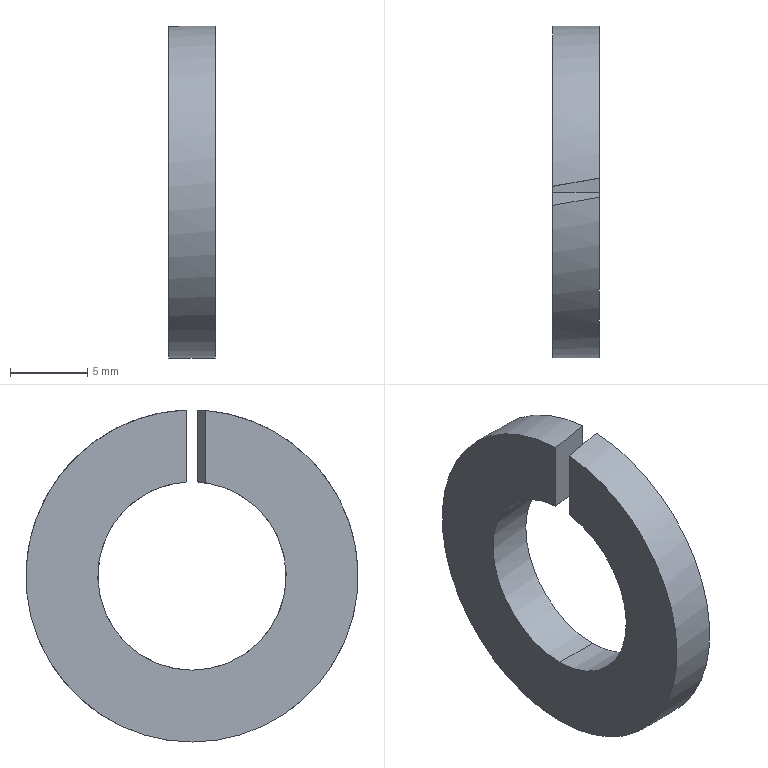Part | STEP file | 0228_318_SSLW12 | 1 solid | 8 faces | box 3 x 21.5 x 21.494 mm | volume 721.153 mm3 | cylinder 4 | plane 4 | commonest cylinder face diameters 12.2 x2 21.5 x2
STEP:
#1=CARTESIAN_POINT('',(0.,0.,0.));
#2=DIRECTION('',(0.,0.,1.));
#3=DIRECTION('',(1.,0.,0.));
#4=AXIS2_PLACEMENT_3D('',#1,#2,#3);
#5=CARTESIAN_POINT('',(-1.5,0.3549,6.09));
#6=VERTEX_POINT('',#5);
#7=CARTESIAN_POINT('',(1.5,0.8839,6.036));
#8=VERTEX_POINT('',#7);
#9=CARTESIAN_POINT('',(-1.5,0.3549,6.09));
#10=CARTESIAN_POINT('',(-0.4959,0.532,6.079));
#11=CARTESIAN_POINT('',(0.5048,0.7084,6.061));
#12=CARTESIAN_POINT('',(1.5,0.8839,6.036));
#13=(BOUNDED_CURVE()B_SPLINE_CURVE(3,(#9,#10,#11,#12),.UNSPECIFIED.,.F.,.F.)B_SPLINE_CURVE_WITH_KNOTS((4,4),(4.771,4.858),.PIECEWISE_BEZIER_KNOTS.)CURVE()GEOMETRIC_REPRESENTATION_ITEM()RATIONAL_B_SPLINE_CURVE((1.,0.9994,0.9994,1.))REPRESENTATION_ITEM(''));
#14=CARTESIAN_POINT('',(0.,0.,0.));
#15=DIRECTION('',(1.,0.,0.));
#16=DIRECTION('',(0.,0.,-1.));
#17=AXIS2_PLACEMENT_3D('',#14,#15,#16);
#18=CYLINDRICAL_SURFACE('',#17,6.1);
#19=CARTESIAN_POINT('',(3.083,-1.5));
#20=CARTESIAN_POINT('',(3.082,-1.454));
#21=CARTESIAN_POINT('',(3.079,-1.363));
#22=CARTESIAN_POINT('',(3.075,-1.226));
#23=CARTESIAN_POINT('',(3.071,-1.09));
#24=CARTESIAN_POINT('',(3.068,-0.9528));
#25=CARTESIAN_POINT('',(3.064,-0.8161));
#26=CARTESIAN_POINT('',(3.06,-0.6794));
#27=CARTESIAN_POINT('',(3.056,-0.5428));
#28=CARTESIAN_POINT('',(3.052,-0.4062));
#29=CARTESIAN_POINT('',(3.048,-0.2696));
#30=CARTESIAN_POINT('',(3.044,-0.1331));
#31=CARTESIAN_POINT('',(3.04,0.003351));
#32=CARTESIAN_POINT('',(3.036,0.1398));
#33=CARTESIAN_POINT('',(3.032,0.2761));
#34=CARTESIAN_POINT('',(3.028,0.4124));
#35=CARTESIAN_POINT('',(3.024,0.5486));
#36=CARTESIAN_POINT('',(3.02,0.6847));
#37=CARTESIAN_POINT('',(3.016,0.8208));
#38=CARTESIAN_POINT('',(3.012,0.9568));
#39=CARTESIAN_POINT('',(3.008,1.093));
#40=CARTESIAN_POINT('',(3.004,1.229));
#41=CARTESIAN_POINT('',(3.,1.364));
#42=CARTESIAN_POINT('',(2.997,1.455));
#43=CARTESIAN_POINT('',(2.996,1.5));
#44=B_SPLINE_CURVE_WITH_KNOTS('',3,(#19,#20,#21,#22,#23,#24,#25,#26,#27,#28,#29,#30,#31,#32,#33,#34,#35,#36,#37,#38,#39,#40,#41,#42,#43),.UNSPECIFIED.,.F.,.F.,(4,1,1,1,1,1,1,1,1,1,1,1,1,1,1,1,1,1,1,1,1,1,4),(4.771,4.775,4.779,4.782,4.786,4.79,4.794,4.798,4.802,4.806,4.81,4.814,4.818,4.822,4.826,4.83,4.834,4.838,4.842,4.846,4.85,4.854,4.858),.QUASI_UNIFORM_KNOTS.);
#45=(GEOMETRIC_REPRESENTATION_CONTEXT(2)PARAMETRIC_REPRESENTATION_CONTEXT()REPRESENTATION_CONTEXT('',''));
#46=DEFINITIONAL_REPRESENTATION('',(#44),#45);
#47=PCURVE('',#18,#46);
#48=CARTESIAN_POINT('',(-3.06,0.07979,0.));
#49=DIRECTION('',(-0.1736,0.9848,0.));
#50=DIRECTION('',(-0.9848,-0.1736,0.));
#51=AXIS2_PLACEMENT_3D('',#48,#49,#50);
#52=PLANE('',#51);
#53=CARTESIAN_POINT('',(-1.584,6.09));
#54=CARTESIAN_POINT('',(-2.604,6.079));
#55=CARTESIAN_POINT('',(-3.62,6.061));
#56=CARTESIAN_POINT('',(-4.631,6.036));
#57=(BOUNDED_CURVE()B_SPLINE_CURVE(3,(#53,#54,#55,#56),.UNSPECIFIED.,.F.,.F.)B_SPLINE_CURVE_WITH_KNOTS((4,4),(4.771,4.858),.PIECEWISE_BEZIER_KNOTS.)CURVE()GEOMETRIC_REPRESENTATION_ITEM()RATIONAL_B_SPLINE_CURVE((1.,0.9994,0.9994,1.))REPRESENTATION_ITEM(''));
#58=(GEOMETRIC_REPRESENTATION_CONTEXT(2)PARAMETRIC_REPRESENTATION_CONTEXT()REPRESENTATION_CONTEXT('',''));
#59=DEFINITIONAL_REPRESENTATION('',(#57),#58);
#60=PCURVE('',#52,#59);
#61=SURFACE_CURVE('',#13,(#47,#60),.PCURVE_S1.);
#62=EDGE_CURVE('',#6,#8,#61,.T.);
#63=ORIENTED_EDGE('',*,*,#62,.T.);
#64=CARTESIAN_POINT('',(1.5,0.,-6.1));
#65=VERTEX_POINT('',#64);
#66=CARTESIAN_POINT('',(1.5,0.,0.));
#67=DIRECTION('',(-1.,0.,0.));
#68=DIRECTION('',(0.,0.,-1.));
#69=AXIS2_PLACEMENT_3D('',#66,#67,#68);
#70=CIRCLE('',#69,6.1);
#71=CARTESIAN_POINT('',(6.283,1.5));
#72=DIRECTION('',(-1.,0.));
#73=VECTOR('',#72,1.);
#74=LINE('',#71,#73);
#75=(GEOMETRIC_REPRESENTATION_CONTEXT(2)PARAMETRIC_REPRESENTATION_CONTEXT()REPRESENTATION_CONTEXT('',''));
#76=DEFINITIONAL_REPRESENTATION('',(#74),#75);
#77=PCURVE('',#18,#76);
#78=CARTESIAN_POINT('',(1.5,8.425,0.));
#79=DIRECTION('',(1.,0.,0.));
#80=DIRECTION('',(0.,0.,-1.));
#81=AXIS2_PLACEMENT_3D('',#78,#79,#80);
#82=PLANE('',#81);
#83=CARTESIAN_POINT('',(6.1,-8.425));
#84=CARTESIAN_POINT('',(6.1,-18.991));
#85=CARTESIAN_POINT('',(-3.05,-13.708));
#86=CARTESIAN_POINT('',(-12.2,-8.425));
#87=CARTESIAN_POINT('',(-3.05,-3.142));
#88=CARTESIAN_POINT('',(6.1,2.141));
#89=CARTESIAN_POINT('',(6.1,-8.425));
#90=(BOUNDED_CURVE()B_SPLINE_CURVE(2,(#83,#84,#85,#86,#87,#88,#89),.UNSPECIFIED.,.T.,.F.)B_SPLINE_CURVE_WITH_KNOTS((1,2,2,2,2,1),(-2.094,0.,2.094,4.189,6.283,8.378),.UNSPECIFIED.)CURVE()GEOMETRIC_REPRESENTATION_ITEM()RATIONAL_B_SPLINE_CURVE((1.,0.5,1.,0.5,1.,0.5,1.))REPRESENTATION_ITEM(''));
#91=(GEOMETRIC_REPRESENTATION_CONTEXT(2)PARAMETRIC_REPRESENTATION_CONTEXT()REPRESENTATION_CONTEXT('',''));
#92=DEFINITIONAL_REPRESENTATION('',(#90),#91);
#93=PCURVE('',#82,#92);
#94=SURFACE_CURVE('',#70,(#77,#93),.PCURVE_S1.);
#95=EDGE_CURVE('',#8,#65,#94,.T.);
#96=ORIENTED_EDGE('',*,*,#95,.T.);
#97=CARTESIAN_POINT('',(-1.5,0.,-6.1));
#98=VERTEX_POINT('',#97);
#99=CARTESIAN_POINT('',(0.,0.,-6.1));
#100=DIRECTION('',(1.,0.,0.));
#101=VECTOR('',#100,1.);
#102=LINE('',#99,#101);
#103=CARTESIAN_POINT('',(0.,0.));
#104=DIRECTION('',(0.,1.));
#105=VECTOR('',#104,1.);
#106=LINE('',#103,#105);
#107=(GEOMETRIC_REPRESENTATION_CONTEXT(2)PARAMETRIC_REPRESENTATION_CONTEXT()REPRESENTATION_CONTEXT('',''));
#108=DEFINITIONAL_REPRESENTATION('',(#106),#107);
#109=PCURVE('',#18,#108);
#110=CARTESIAN_POINT('',(0.,0.,0.));
#111=DIRECTION('',(1.,0.,0.));
#112=DIRECTION('',(0.,0.,-1.));
#113=AXIS2_PLACEMENT_3D('',#110,#111,#112);
#114=CYLINDRICAL_SURFACE('',#113,6.1);
#115=CARTESIAN_POINT('',(6.283,0.));
#116=DIRECTION('',(0.,1.));
#117=VECTOR('',#116,1.);
#118=LINE('',#115,#117);
#119=(GEOMETRIC_REPRESENTATION_CONTEXT(2)PARAMETRIC_REPRESENTATION_CONTEXT()REPRESENTATION_CONTEXT('',''));
#120=DEFINITIONAL_REPRESENTATION('',(#118),#119);
#121=PCURVE('',#114,#120);
#122=SURFACE_CURVE('',#102,(#109,#121),.PCURVE_S1.);
#123=EDGE_CURVE('',#98,#65,#122,.T.);
#124=ORIENTED_EDGE('',*,*,#123,.F.);
#125=CARTESIAN_POINT('',(-1.5,0.,0.));
#126=DIRECTION('',(1.,0.,0.));
#127=DIRECTION('',(0.,0.,-1.));
#128=AXIS2_PLACEMENT_3D('',#125,#126,#127);
#129=CIRCLE('',#128,6.1);
#130=CARTESIAN_POINT('',(0.,-1.5));
#131=DIRECTION('',(1.,0.));
#132=VECTOR('',#131,1.);
#133=LINE('',#130,#132);
#134=(GEOMETRIC_REPRESENTATION_CONTEXT(2)PARAMETRIC_REPRESENTATION_CONTEXT()REPRESENTATION_CONTEXT('',''));
#135=DEFINITIONAL_REPRESENTATION('',(#133),#134);
#136=PCURVE('',#18,#135);
#137=CARTESIAN_POINT('',(-1.5,8.425,0.));
#138=DIRECTION('',(-1.,0.,0.));
#139=DIRECTION('',(0.,0.,1.));
#140=AXIS2_PLACEMENT_3D('',#137,#138,#139);
#141=PLANE('',#140);
#142=CARTESIAN_POINT('',(-6.1,-8.425));
#143=CARTESIAN_POINT('',(-6.1,2.141));
#144=CARTESIAN_POINT('',(3.05,-3.142));
#145=CARTESIAN_POINT('',(12.2,-8.425));
#146=CARTESIAN_POINT('',(3.05,-13.708));
#147=CARTESIAN_POINT('',(-6.1,-18.991));
#148=CARTESIAN_POINT('',(-6.1,-8.425));
#149=(BOUNDED_CURVE()B_SPLINE_CURVE(2,(#142,#143,#144,#145,#146,#147,#148),.UNSPECIFIED.,.T.,.F.)B_SPLINE_CURVE_WITH_KNOTS((1,2,2,2,2,1),(-2.094,0.,2.094,4.189,6.283,8.378),.UNSPECIFIED.)CURVE()GEOMETRIC_REPRESENTATION_ITEM()RATIONAL_B_SPLINE_CURVE((1.,0.5,1.,0.5,1.,0.5,1.))REPRESENTATION_ITEM(''));
#150=(GEOMETRIC_REPRESENTATION_CONTEXT(2)PARAMETRIC_REPRESENTATION_CONTEXT()REPRESENTATION_CONTEXT('',''));
#151=DEFINITIONAL_REPRESENTATION('',(#149),#150);
#152=PCURVE('',#141,#151);
#153=SURFACE_CURVE('',#129,(#136,#152),.PCURVE_S1.);
#154=EDGE_CURVE('',#98,#6,#153,.T.);
#155=ORIENTED_EDGE('',*,*,#154,.T.);
#156=EDGE_LOOP('',(#63,#96,#124,#155));
#157=FACE_BOUND('',#156,.F.);
#158=ADVANCED_FACE('',(#157),#18,.F.);
#159=CARTESIAN_POINT('',(-1.5,0.,-10.75));
#160=VERTEX_POINT('',#159);
#161=CARTESIAN_POINT('',(-1.5,-0.8839,10.714));
#162=VERTEX_POINT('',#161);
#163=CARTESIAN_POINT('',(-1.5,0.,0.));
#164=DIRECTION('',(-1.,0.,0.));
#165=DIRECTION('',(0.,0.,-1.));
#166=AXIS2_PLACEMENT_3D('',#163,#164,#165);
#167=CIRCLE('',#166,10.75);
#168=CARTESIAN_POINT('',(0.,0.,0.));
#169=DIRECTION('',(1.,0.,0.));
#170=DIRECTION('',(0.,0.,-1.));
#171=AXIS2_PLACEMENT_3D('',#168,#169,#170);
#172=CYLINDRICAL_SURFACE('',#171,10.75);
#173=CARTESIAN_POINT('',(6.283,-1.5));
#174=DIRECTION('',(-1.,0.));
#175=VECTOR('',#174,1.);
#176=LINE('',#173,#175);
#177=(GEOMETRIC_REPRESENTATION_CONTEXT(2)PARAMETRIC_REPRESENTATION_CONTEXT()REPRESENTATION_CONTEXT('',''));
#178=DEFINITIONAL_REPRESENTATION('',(#176),#177);
#179=PCURVE('',#172,#178);
#180=CARTESIAN_POINT('',(0.,-8.425));
#181=DIRECTION('',(-1.,0.));
#182=AXIS2_PLACEMENT_2D('',#180,#181);
#183=CIRCLE('',#182,10.75);
#184=(GEOMETRIC_REPRESENTATION_CONTEXT(2)PARAMETRIC_REPRESENTATION_CONTEXT()REPRESENTATION_CONTEXT('',''));
#185=DEFINITIONAL_REPRESENTATION('',(#183),#184);
#186=PCURVE('',#141,#185);
#187=SURFACE_CURVE('',#167,(#179,#186),.PCURVE_S1.);
#188=EDGE_CURVE('',#160,#162,#187,.T.);
#189=ORIENTED_EDGE('',*,*,#188,.F.);
#190=CARTESIAN_POINT('',(1.5,0.,-10.75));
#191=VERTEX_POINT('',#190);
#192=CARTESIAN_POINT('',(0.,0.,-10.75));
#193=DIRECTION('',(1.,0.,0.));
#194=VECTOR('',#193,1.);
#195=LINE('',#192,#194);
#196=CARTESIAN_POINT('',(6.283,0.));
#197=DIRECTION('',(0.,1.));
#198=VECTOR('',#197,1.);
#199=LINE('',#196,#198);
#200=(GEOMETRIC_REPRESENTATION_CONTEXT(2)PARAMETRIC_REPRESENTATION_CONTEXT()REPRESENTATION_CONTEXT('',''));
#201=DEFINITIONAL_REPRESENTATION('',(#199),#200);
#202=PCURVE('',#172,#201);
#203=CARTESIAN_POINT('',(0.,0.,0.));
#204=DIRECTION('',(1.,0.,0.));
#205=DIRECTION('',(0.,0.,-1.));
#206=AXIS2_PLACEMENT_3D('',#203,#204,#205);
#207=CYLINDRICAL_SURFACE('',#206,10.75);
#208=CARTESIAN_POINT('',(0.,0.));
#209=DIRECTION('',(0.,1.));
#210=VECTOR('',#209,1.);
#211=LINE('',#208,#210);
#212=(GEOMETRIC_REPRESENTATION_CONTEXT(2)PARAMETRIC_REPRESENTATION_CONTEXT()REPRESENTATION_CONTEXT('',''));
#213=DEFINITIONAL_REPRESENTATION('',(#211),#212);
#214=PCURVE('',#207,#213);
#215=SURFACE_CURVE('',#195,(#202,#214),.PCURVE_S1.);
#216=EDGE_CURVE('',#160,#191,#215,.T.);
#217=ORIENTED_EDGE('',*,*,#216,.T.);
#218=CARTESIAN_POINT('',(1.5,-0.3549,10.744));
#219=VERTEX_POINT('',#218);
#220=CARTESIAN_POINT('',(1.5,0.,0.));
#221=DIRECTION('',(-1.,0.,0.));
#222=DIRECTION('',(0.,0.,-1.));
#223=AXIS2_PLACEMENT_3D('',#220,#221,#222);
#224=CIRCLE('',#223,10.75);
#225=CARTESIAN_POINT('',(6.283,1.5));
#226=DIRECTION('',(-1.,0.));
#227=VECTOR('',#226,1.);
#228=LINE('',#225,#227);
#229=(GEOMETRIC_REPRESENTATION_CONTEXT(2)PARAMETRIC_REPRESENTATION_CONTEXT()REPRESENTATION_CONTEXT('',''));
#230=DEFINITIONAL_REPRESENTATION('',(#228),#229);
#231=PCURVE('',#172,#230);
#232=CARTESIAN_POINT('',(10.75,-8.425));
#233=CARTESIAN_POINT('',(10.75,-27.045));
#234=CARTESIAN_POINT('',(-5.375,-17.735));
#235=CARTESIAN_POINT('',(-21.5,-8.425));
#236=CARTESIAN_POINT('',(-5.375,0.8848));
#237=CARTESIAN_POINT('',(10.75,10.195));
#238=CARTESIAN_POINT('',(10.75,-8.425));
#239=(BOUNDED_CURVE()B_SPLINE_CURVE(2,(#232,#233,#234,#235,#236,#237,#238),.UNSPECIFIED.,.T.,.F.)B_SPLINE_CURVE_WITH_KNOTS((1,2,2,2,2,1),(-2.094,0.,2.094,4.189,6.283,8.378),.UNSPECIFIED.)CURVE()GEOMETRIC_REPRESENTATION_ITEM()RATIONAL_B_SPLINE_CURVE((1.,0.5,1.,0.5,1.,0.5,1.))REPRESENTATION_ITEM(''));
#240=(GEOMETRIC_REPRESENTATION_CONTEXT(2)PARAMETRIC_REPRESENTATION_CONTEXT()REPRESENTATION_CONTEXT('',''));
#241=DEFINITIONAL_REPRESENTATION('',(#239),#240);
#242=PCURVE('',#82,#241);
#243=SURFACE_CURVE('',#224,(#231,#242),.PCURVE_S1.);
#244=EDGE_CURVE('',#191,#219,#243,.T.);
#245=ORIENTED_EDGE('',*,*,#244,.T.);
#246=CARTESIAN_POINT('',(1.5,-0.3549,10.744));
#247=CARTESIAN_POINT('',(0.4987,-0.5315,10.738));
#248=CARTESIAN_POINT('',(-0.5015,-0.7078,10.728));
#249=CARTESIAN_POINT('',(-1.5,-0.8839,10.714));
#250=(BOUNDED_CURVE()B_SPLINE_CURVE(3,(#246,#247,#248,#249),.UNSPECIFIED.,.F.,.F.)B_SPLINE_CURVE_WITH_KNOTS((4,4),(1.604,1.653),.PIECEWISE_BEZIER_KNOTS.)CURVE()GEOMETRIC_REPRESENTATION_ITEM()RATIONAL_B_SPLINE_CURVE((1.,0.9998,0.9998,1.))REPRESENTATION_ITEM(''));
#251=CARTESIAN_POINT('',(3.175,1.5));
#252=CARTESIAN_POINT('',(3.175,1.454));
#253=CARTESIAN_POINT('',(3.177,1.363));
#254=CARTESIAN_POINT('',(3.179,1.227));
#255=CARTESIAN_POINT('',(3.181,1.09));
#256=CARTESIAN_POINT('',(3.184,0.954));
#257=CARTESIAN_POINT('',(3.186,0.8175));
#258=CARTESIAN_POINT('',(3.188,0.6811));
#259=CARTESIAN_POINT('',(3.19,0.5446));
#260=CARTESIAN_POINT('',(3.193,0.4082));
#261=CARTESIAN_POINT('',(3.195,0.2717));
#262=CARTESIAN_POINT('',(3.197,0.1353));
#263=CARTESIAN_POINT('',(3.199,-0.00107));
#264=CARTESIAN_POINT('',(3.202,-0.1374));
#265=CARTESIAN_POINT('',(3.204,-0.2738));
#266=CARTESIAN_POINT('',(3.206,-0.4101));
#267=CARTESIAN_POINT('',(3.208,-0.5465));
#268=CARTESIAN_POINT('',(3.21,-0.6828));
#269=CARTESIAN_POINT('',(3.213,-0.819));
#270=CARTESIAN_POINT('',(3.215,-0.9553));
#271=CARTESIAN_POINT('',(3.217,-1.091));
#272=CARTESIAN_POINT('',(3.219,-1.228));
#273=CARTESIAN_POINT('',(3.222,-1.364));
#274=CARTESIAN_POINT('',(3.223,-1.455));
#275=CARTESIAN_POINT('',(3.224,-1.5));
#276=B_SPLINE_CURVE_WITH_KNOTS('',3,(#251,#252,#253,#254,#255,#256,#257,#258,#259,#260,#261,#262,#263,#264,#265,#266,#267,#268,#269,#270,#271,#272,#273,#274,#275),.UNSPECIFIED.,.F.,.F.,(4,1,1,1,1,1,1,1,1,1,1,1,1,1,1,1,1,1,1,1,1,1,4),(1.604,1.606,1.608,1.611,1.613,1.615,1.617,1.62,1.622,1.624,1.626,1.628,1.631,1.633,1.635,1.637,1.64,1.642,1.644,1.646,1.649,1.651,1.653),.QUASI_UNIFORM_KNOTS.);
#277=(GEOMETRIC_REPRESENTATION_CONTEXT(2)PARAMETRIC_REPRESENTATION_CONTEXT()REPRESENTATION_CONTEXT('',''));
#278=DEFINITIONAL_REPRESENTATION('',(#276),#277);
#279=PCURVE('',#172,#278);
#280=CARTESIAN_POINT('',(3.06,-0.07979,0.));
#281=DIRECTION('',(0.1736,-0.9848,0.));
#282=DIRECTION('',(0.9848,0.1736,0.));
#283=AXIS2_PLACEMENT_3D('',#280,#281,#282);
#284=PLANE('',#283);
#285=CARTESIAN_POINT('',(-1.584,10.744));
#286=CARTESIAN_POINT('',(-2.601,10.738));
#287=CARTESIAN_POINT('',(-3.617,10.728));
#288=CARTESIAN_POINT('',(-4.631,10.714));
#289=(BOUNDED_CURVE()B_SPLINE_CURVE(3,(#285,#286,#287,#288),.UNSPECIFIED.,.F.,.F.)B_SPLINE_CURVE_WITH_KNOTS((4,4),(1.604,1.653),.PIECEWISE_BEZIER_KNOTS.)CURVE()GEOMETRIC_REPRESENTATION_ITEM()RATIONAL_B_SPLINE_CURVE((1.,0.9998,0.9998,1.))REPRESENTATION_ITEM(''));
#290=(GEOMETRIC_REPRESENTATION_CONTEXT(2)PARAMETRIC_REPRESENTATION_CONTEXT()REPRESENTATION_CONTEXT('',''));
#291=DEFINITIONAL_REPRESENTATION('',(#289),#290);
#292=PCURVE('',#284,#291);
#293=SURFACE_CURVE('',#250,(#279,#292),.PCURVE_S1.);
#294=EDGE_CURVE('',#219,#162,#293,.T.);
#295=ORIENTED_EDGE('',*,*,#294,.T.);
#296=EDGE_LOOP('',(#189,#217,#245,#295));
#297=FACE_BOUND('',#296,.T.);
#298=ADVANCED_FACE('',(#297),#172,.T.);
#299=CARTESIAN_POINT('',(-1.5,-0.8839,6.036));
#300=VERTEX_POINT('',#299);
#301=CARTESIAN_POINT('',(-1.5,0.,0.));
#302=DIRECTION('',(1.,0.,0.));
#303=DIRECTION('',(0.,0.,-1.));
#304=AXIS2_PLACEMENT_3D('',#301,#302,#303);
#305=CIRCLE('',#304,6.1);
#306=CARTESIAN_POINT('',(-6.1,-8.425));
#307=CARTESIAN_POINT('',(-6.1,2.141));
#308=CARTESIAN_POINT('',(3.05,-3.142));
#309=CARTESIAN_POINT('',(12.2,-8.425));
#310=CARTESIAN_POINT('',(3.05,-13.708));
#311=CARTESIAN_POINT('',(-6.1,-18.991));
#312=CARTESIAN_POINT('',(-6.1,-8.425));
#313=(BOUNDED_CURVE()B_SPLINE_CURVE(2,(#306,#307,#308,#309,#310,#311,#312),.UNSPECIFIED.,.T.,.F.)B_SPLINE_CURVE_WITH_KNOTS((1,2,2,2,2,1),(-2.094,0.,2.094,4.189,6.283,8.378),.UNSPECIFIED.)CURVE()GEOMETRIC_REPRESENTATION_ITEM()RATIONAL_B_SPLINE_CURVE((1.,0.5,1.,0.5,1.,0.5,1.))REPRESENTATION_ITEM(''));
#314=(GEOMETRIC_REPRESENTATION_CONTEXT(2)PARAMETRIC_REPRESENTATION_CONTEXT()REPRESENTATION_CONTEXT('',''));
#315=DEFINITIONAL_REPRESENTATION('',(#313),#314);
#316=PCURVE('',#141,#315);
#317=CARTESIAN_POINT('',(0.,-1.5));
#318=DIRECTION('',(1.,0.));
#319=VECTOR('',#318,1.);
#320=LINE('',#317,#319);
#321=(GEOMETRIC_REPRESENTATION_CONTEXT(2)PARAMETRIC_REPRESENTATION_CONTEXT()REPRESENTATION_CONTEXT('',''));
#322=DEFINITIONAL_REPRESENTATION('',(#320),#321);
#323=PCURVE('',#114,#322);
#324=SURFACE_CURVE('',#305,(#316,#323),.PCURVE_S1.);
#325=EDGE_CURVE('',#300,#98,#324,.T.);
#326=ORIENTED_EDGE('',*,*,#325,.T.);
#327=ORIENTED_EDGE('',*,*,#154,.T.);
#328=CARTESIAN_POINT('',(-1.5,0.3549,10.744));
#329=VERTEX_POINT('',#328);
#330=CARTESIAN_POINT('',(-1.5,0.3549,0.));
#331=DIRECTION('',(0.,0.,1.));
#332=VECTOR('',#331,1.);
#333=LINE('',#330,#332);
#334=CARTESIAN_POINT('',(0.,-8.07));
#335=DIRECTION('',(1.,0.));
#336=VECTOR('',#335,1.);
#337=LINE('',#334,#336);
#338=(GEOMETRIC_REPRESENTATION_CONTEXT(2)PARAMETRIC_REPRESENTATION_CONTEXT()REPRESENTATION_CONTEXT('',''));
#339=DEFINITIONAL_REPRESENTATION('',(#337),#338);
#340=PCURVE('',#141,#339);
#341=CARTESIAN_POINT('',(-1.584,0.));
#342=DIRECTION('',(0.,1.));
#343=VECTOR('',#342,1.);
#344=LINE('',#341,#343);
#345=(GEOMETRIC_REPRESENTATION_CONTEXT(2)PARAMETRIC_REPRESENTATION_CONTEXT()REPRESENTATION_CONTEXT('',''));
#346=DEFINITIONAL_REPRESENTATION('',(#344),#345);
#347=PCURVE('',#52,#346);
#348=SURFACE_CURVE('',#333,(#340,#347),.PCURVE_S1.);
#349=EDGE_CURVE('',#6,#329,#348,.T.);
#350=ORIENTED_EDGE('',*,*,#349,.T.);
#351=CARTESIAN_POINT('',(-1.5,0.,0.));
#352=DIRECTION('',(-1.,0.,0.));
#353=DIRECTION('',(0.,0.,-1.));
#354=AXIS2_PLACEMENT_3D('',#351,#352,#353);
#355=CIRCLE('',#354,10.75);
#356=CARTESIAN_POINT('',(0.,-8.425));
#357=DIRECTION('',(-1.,0.));
#358=AXIS2_PLACEMENT_2D('',#356,#357);
#359=CIRCLE('',#358,10.75);
#360=(GEOMETRIC_REPRESENTATION_CONTEXT(2)PARAMETRIC_REPRESENTATION_CONTEXT()REPRESENTATION_CONTEXT('',''));
#361=DEFINITIONAL_REPRESENTATION('',(#359),#360);
#362=PCURVE('',#141,#361);
#363=CARTESIAN_POINT('',(6.283,-1.5));
#364=DIRECTION('',(-1.,0.));
#365=VECTOR('',#364,1.);
#366=LINE('',#363,#365);
#367=(GEOMETRIC_REPRESENTATION_CONTEXT(2)PARAMETRIC_REPRESENTATION_CONTEXT()REPRESENTATION_CONTEXT('',''));
#368=DEFINITIONAL_REPRESENTATION('',(#366),#367);
#369=PCURVE('',#207,#368);
#370=SURFACE_CURVE('',#355,(#362,#369),.PCURVE_S1.);
#371=EDGE_CURVE('',#329,#160,#370,.T.);
#372=ORIENTED_EDGE('',*,*,#371,.T.);
#373=ORIENTED_EDGE('',*,*,#188,.T.);
#374=CARTESIAN_POINT('',(-1.5,-0.8839,0.));
#375=DIRECTION('',(0.,0.,-1.));
#376=VECTOR('',#375,1.);
#377=LINE('',#374,#376);
#378=CARTESIAN_POINT('',(0.,-9.309));
#379=DIRECTION('',(-1.,0.));
#380=VECTOR('',#379,1.);
#381=LINE('',#378,#380);
#382=(GEOMETRIC_REPRESENTATION_CONTEXT(2)PARAMETRIC_REPRESENTATION_CONTEXT()REPRESENTATION_CONTEXT('',''));
#383=DEFINITIONAL_REPRESENTATION('',(#381),#382);
#384=PCURVE('',#141,#383);
#385=CARTESIAN_POINT('',(-4.631,0.));
#386=DIRECTION('',(0.,-1.));
#387=VECTOR('',#386,1.);
#388=LINE('',#385,#387);
#389=(GEOMETRIC_REPRESENTATION_CONTEXT(2)PARAMETRIC_REPRESENTATION_CONTEXT()REPRESENTATION_CONTEXT('',''));
#390=DEFINITIONAL_REPRESENTATION('',(#388),#389);
#391=PCURVE('',#284,#390);
#392=SURFACE_CURVE('',#377,(#384,#391),.PCURVE_S1.);
#393=EDGE_CURVE('',#162,#300,#392,.T.);
#394=ORIENTED_EDGE('',*,*,#393,.T.);
#395=EDGE_LOOP('',(#326,#327,#350,#372,#373,#394));
#396=FACE_BOUND('',#395,.T.);
#397=ADVANCED_FACE('',(#396),#141,.T.);
#398=CARTESIAN_POINT('',(1.5,-0.3549,6.09));
#399=VERTEX_POINT('',#398);
#400=CARTESIAN_POINT('',(1.5,0.,0.));
#401=DIRECTION('',(-1.,0.,0.));
#402=DIRECTION('',(0.,0.,-1.));
#403=AXIS2_PLACEMENT_3D('',#400,#401,#402);
#404=CIRCLE('',#403,6.1);
#405=CARTESIAN_POINT('',(6.283,1.5));
#406=DIRECTION('',(-1.,0.));
#407=VECTOR('',#406,1.);
#408=LINE('',#405,#407);
#409=(GEOMETRIC_REPRESENTATION_CONTEXT(2)PARAMETRIC_REPRESENTATION_CONTEXT()REPRESENTATION_CONTEXT('',''));
#410=DEFINITIONAL_REPRESENTATION('',(#408),#409);
#411=PCURVE('',#114,#410);
#412=CARTESIAN_POINT('',(6.1,-8.425));
#413=CARTESIAN_POINT('',(6.1,-18.991));
#414=CARTESIAN_POINT('',(-3.05,-13.708));
#415=CARTESIAN_POINT('',(-12.2,-8.425));
#416=CARTESIAN_POINT('',(-3.05,-3.142));
#417=CARTESIAN_POINT('',(6.1,2.141));
#418=CARTESIAN_POINT('',(6.1,-8.425));
#419=(BOUNDED_CURVE()B_SPLINE_CURVE(2,(#412,#413,#414,#415,#416,#417,#418),.UNSPECIFIED.,.T.,.F.)B_SPLINE_CURVE_WITH_KNOTS((1,2,2,2,2,1),(-2.094,0.,2.094,4.189,6.283,8.378),.UNSPECIFIED.)CURVE()GEOMETRIC_REPRESENTATION_ITEM()RATIONAL_B_SPLINE_CURVE((1.,0.5,1.,0.5,1.,0.5,1.))REPRESENTATION_ITEM(''));
#420=(GEOMETRIC_REPRESENTATION_CONTEXT(2)PARAMETRIC_REPRESENTATION_CONTEXT()REPRESENTATION_CONTEXT('',''));
#421=DEFINITIONAL_REPRESENTATION('',(#419),#420);
#422=PCURVE('',#82,#421);
#423=SURFACE_CURVE('',#404,(#411,#422),.PCURVE_S1.);
#424=EDGE_CURVE('',#65,#399,#423,.T.);
#425=ORIENTED_EDGE('',*,*,#424,.T.);
#426=CARTESIAN_POINT('',(1.5,-0.3549,6.09));
#427=CARTESIAN_POINT('',(0.4959,-0.532,6.079));
#428=CARTESIAN_POINT('',(-0.5048,-0.7084,6.061));
#429=CARTESIAN_POINT('',(-1.5,-0.8839,6.036));
#430=(BOUNDED_CURVE()B_SPLINE_CURVE(3,(#426,#427,#428,#429),.UNSPECIFIED.,.F.,.F.)B_SPLINE_CURVE_WITH_KNOTS((4,4),(1.629,1.716),.PIECEWISE_BEZIER_KNOTS.)CURVE()GEOMETRIC_REPRESENTATION_ITEM()RATIONAL_B_SPLINE_CURVE((1.,0.9994,0.9994,1.))REPRESENTATION_ITEM(''));
#431=CARTESIAN_POINT('',(3.2,1.5));
#432=CARTESIAN_POINT('',(3.201,1.454));
#433=CARTESIAN_POINT('',(3.204,1.363));
#434=CARTESIAN_POINT('',(3.208,1.226));
#435=CARTESIAN_POINT('',(3.212,1.09));
#436=CARTESIAN_POINT('',(3.216,0.9528));
#437=CARTESIAN_POINT('',(3.22,0.8161));
#438=CARTESIAN_POINT('',(3.224,0.6794));
#439=CARTESIAN_POINT('',(3.228,0.5428));
#440=CARTESIAN_POINT('',(3.232,0.4062));
#441=CARTESIAN_POINT('',(3.235,0.2696));
#442=CARTESIAN_POINT('',(3.239,0.1331));
#443=CARTESIAN_POINT('',(3.243,-0.003351));
#444=CARTESIAN_POINT('',(3.247,-0.1398));
#445=CARTESIAN_POINT('',(3.251,-0.2761));
#446=CARTESIAN_POINT('',(3.255,-0.4124));
#447=CARTESIAN_POINT('',(3.259,-0.5486));
#448=CARTESIAN_POINT('',(3.263,-0.6847));
#449=CARTESIAN_POINT('',(3.267,-0.8208));
#450=CARTESIAN_POINT('',(3.271,-0.9568));
#451=CARTESIAN_POINT('',(3.275,-1.093));
#452=CARTESIAN_POINT('',(3.279,-1.229));
#453=CARTESIAN_POINT('',(3.283,-1.364));
#454=CARTESIAN_POINT('',(3.286,-1.455));
#455=CARTESIAN_POINT('',(3.287,-1.5));
#456=B_SPLINE_CURVE_WITH_KNOTS('',3,(#431,#432,#433,#434,#435,#436,#437,#438,#439,#440,#441,#442,#443,#444,#445,#446,#447,#448,#449,#450,#451,#452,#453,#454,#455),.UNSPECIFIED.,.F.,.F.,(4,1,1,1,1,1,1,1,1,1,1,1,1,1,1,1,1,1,1,1,1,1,4),(1.629,1.633,1.637,1.641,1.645,1.649,1.653,1.657,1.661,1.665,1.669,1.673,1.677,1.681,1.685,1.688,1.692,1.696,1.7,1.704,1.708,1.712,1.716),.QUASI_UNIFORM_KNOTS.);
#457=(GEOMETRIC_REPRESENTATION_CONTEXT(2)PARAMETRIC_REPRESENTATION_CONTEXT()REPRESENTATION_CONTEXT('',''));
#458=DEFINITIONAL_REPRESENTATION('',(#456),#457);
#459=PCURVE('',#114,#458);
#460=CARTESIAN_POINT('',(-1.584,6.09));
#461=CARTESIAN_POINT('',(-2.604,6.079));
#462=CARTESIAN_POINT('',(-3.62,6.061));
#463=CARTESIAN_POINT('',(-4.631,6.036));
#464=(BOUNDED_CURVE()B_SPLINE_CURVE(3,(#460,#461,#462,#463),.UNSPECIFIED.,.F.,.F.)B_SPLINE_CURVE_WITH_KNOTS((4,4),(1.629,1.716),.PIECEWISE_BEZIER_KNOTS.)CURVE()GEOMETRIC_REPRESENTATION_ITEM()RATIONAL_B_SPLINE_CURVE((1.,0.9994,0.9994,1.))REPRESENTATION_ITEM(''));
#465=(GEOMETRIC_REPRESENTATION_CONTEXT(2)PARAMETRIC_REPRESENTATION_CONTEXT()REPRESENTATION_CONTEXT('',''));
#466=DEFINITIONAL_REPRESENTATION('',(#464),#465);
#467=PCURVE('',#284,#466);
#468=SURFACE_CURVE('',#430,(#459,#467),.PCURVE_S1.);
#469=EDGE_CURVE('',#399,#300,#468,.T.);
#470=ORIENTED_EDGE('',*,*,#469,.T.);
#471=ORIENTED_EDGE('',*,*,#325,.T.);
#472=ORIENTED_EDGE('',*,*,#123,.T.);
#473=EDGE_LOOP('',(#425,#470,#471,#472));
#474=FACE_BOUND('',#473,.F.);
#475=ADVANCED_FACE('',(#474),#114,.F.);
#476=ORIENTED_EDGE('',*,*,#469,.T.);
#477=ORIENTED_EDGE('',*,*,#393,.F.);
#478=ORIENTED_EDGE('',*,*,#294,.F.);
#479=CARTESIAN_POINT('',(1.5,-0.3549,0.));
#480=DIRECTION('',(0.,0.,1.));
#481=VECTOR('',#480,1.);
#482=LINE('',#479,#481);
#483=CARTESIAN_POINT('',(-1.584,0.));
#484=DIRECTION('',(0.,1.));
#485=VECTOR('',#484,1.);
#486=LINE('',#483,#485);
#487=(GEOMETRIC_REPRESENTATION_CONTEXT(2)PARAMETRIC_REPRESENTATION_CONTEXT()REPRESENTATION_CONTEXT('',''));
#488=DEFINITIONAL_REPRESENTATION('',(#486),#487);
#489=PCURVE('',#284,#488);
#490=CARTESIAN_POINT('',(0.,-8.78));
#491=DIRECTION('',(-1.,0.));
#492=VECTOR('',#491,1.);
#493=LINE('',#490,#492);
#494=(GEOMETRIC_REPRESENTATION_CONTEXT(2)PARAMETRIC_REPRESENTATION_CONTEXT()REPRESENTATION_CONTEXT('',''));
#495=DEFINITIONAL_REPRESENTATION('',(#493),#494);
#496=PCURVE('',#82,#495);
#497=SURFACE_CURVE('',#482,(#489,#496),.PCURVE_S1.);
#498=EDGE_CURVE('',#399,#219,#497,.T.);
#499=ORIENTED_EDGE('',*,*,#498,.F.);
#500=EDGE_LOOP('',(#476,#477,#478,#499));
#501=FACE_BOUND('',#500,.T.);
#502=ADVANCED_FACE('',(#501),#284,.F.);
#503=ORIENTED_EDGE('',*,*,#216,.F.);
#504=ORIENTED_EDGE('',*,*,#371,.F.);
#505=CARTESIAN_POINT('',(1.5,0.8839,10.714));
#506=VERTEX_POINT('',#505);
#507=CARTESIAN_POINT('',(-1.5,0.3549,10.744));
#508=CARTESIAN_POINT('',(-0.4987,0.5315,10.738));
#509=CARTESIAN_POINT('',(0.5015,0.7078,10.728));
#510=CARTESIAN_POINT('',(1.5,0.8839,10.714));
#511=(BOUNDED_CURVE()B_SPLINE_CURVE(3,(#507,#508,#509,#510),.UNSPECIFIED.,.F.,.F.)B_SPLINE_CURVE_WITH_KNOTS((4,4),(4.745,4.795),.PIECEWISE_BEZIER_KNOTS.)CURVE()GEOMETRIC_REPRESENTATION_ITEM()RATIONAL_B_SPLINE_CURVE((1.,0.9998,0.9998,1.))REPRESENTATION_ITEM(''));
#512=CARTESIAN_POINT('',(3.109,-1.5));
#513=CARTESIAN_POINT('',(3.108,-1.454));
#514=CARTESIAN_POINT('',(3.106,-1.363));
#515=CARTESIAN_POINT('',(3.104,-1.227));
#516=CARTESIAN_POINT('',(3.102,-1.09));
#517=CARTESIAN_POINT('',(3.1,-0.954));
#518=CARTESIAN_POINT('',(3.097,-0.8175));
#519=CARTESIAN_POINT('',(3.095,-0.6811));
#520=CARTESIAN_POINT('',(3.093,-0.5446));
#521=CARTESIAN_POINT('',(3.091,-0.4082));
#522=CARTESIAN_POINT('',(3.088,-0.2717));
#523=CARTESIAN_POINT('',(3.086,-0.1353));
#524=CARTESIAN_POINT('',(3.084,0.00107));
#525=CARTESIAN_POINT('',(3.082,0.1374));
#526=CARTESIAN_POINT('',(3.079,0.2738));
#527=CARTESIAN_POINT('',(3.077,0.4101));
#528=CARTESIAN_POINT('',(3.075,0.5465));
#529=CARTESIAN_POINT('',(3.073,0.6828));
#530=CARTESIAN_POINT('',(3.07,0.819));
#531=CARTESIAN_POINT('',(3.068,0.9553));
#532=CARTESIAN_POINT('',(3.066,1.091));
#533=CARTESIAN_POINT('',(3.064,1.228));
#534=CARTESIAN_POINT('',(3.062,1.364));
#535=CARTESIAN_POINT('',(3.06,1.455));
#536=CARTESIAN_POINT('',(3.059,1.5));
#537=B_SPLINE_CURVE_WITH_KNOTS('',3,(#512,#513,#514,#515,#516,#517,#518,#519,#520,#521,#522,#523,#524,#525,#526,#527,#528,#529,#530,#531,#532,#533,#534,#535,#536),.UNSPECIFIED.,.F.,.F.,(4,1,1,1,1,1,1,1,1,1,1,1,1,1,1,1,1,1,1,1,1,1,4),(4.745,4.748,4.75,4.752,4.754,4.757,4.759,4.761,4.763,4.766,4.768,4.77,4.772,4.775,4.777,4.779,4.781,4.784,4.786,4.788,4.79,4.792,4.795),.QUASI_UNIFORM_KNOTS.);
#538=(GEOMETRIC_REPRESENTATION_CONTEXT(2)PARAMETRIC_REPRESENTATION_CONTEXT()REPRESENTATION_CONTEXT('',''));
#539=DEFINITIONAL_REPRESENTATION('',(#537),#538);
#540=PCURVE('',#207,#539);
#541=CARTESIAN_POINT('',(-1.584,10.744));
#542=CARTESIAN_POINT('',(-2.601,10.738));
#543=CARTESIAN_POINT('',(-3.617,10.728));
#544=CARTESIAN_POINT('',(-4.631,10.714));
#545=(BOUNDED_CURVE()B_SPLINE_CURVE(3,(#541,#542,#543,#544),.UNSPECIFIED.,.F.,.F.)B_SPLINE_CURVE_WITH_KNOTS((4,4),(4.745,4.795),.PIECEWISE_BEZIER_KNOTS.)CURVE()GEOMETRIC_REPRESENTATION_ITEM()RATIONAL_B_SPLINE_CURVE((1.,0.9998,0.9998,1.))REPRESENTATION_ITEM(''));
#546=(GEOMETRIC_REPRESENTATION_CONTEXT(2)PARAMETRIC_REPRESENTATION_CONTEXT()REPRESENTATION_CONTEXT('',''));
#547=DEFINITIONAL_REPRESENTATION('',(#545),#546);
#548=PCURVE('',#52,#547);
#549=SURFACE_CURVE('',#511,(#540,#548),.PCURVE_S1.);
#550=EDGE_CURVE('',#329,#506,#549,.T.);
#551=ORIENTED_EDGE('',*,*,#550,.T.);
#552=CARTESIAN_POINT('',(1.5,0.,0.));
#553=DIRECTION('',(-1.,0.,0.));
#554=DIRECTION('',(0.,0.,-1.));
#555=AXIS2_PLACEMENT_3D('',#552,#553,#554);
#556=CIRCLE('',#555,10.75);
#557=CARTESIAN_POINT('',(6.283,1.5));
#558=DIRECTION('',(-1.,0.));
#559=VECTOR('',#558,1.);
#560=LINE('',#557,#559);
#561=(GEOMETRIC_REPRESENTATION_CONTEXT(2)PARAMETRIC_REPRESENTATION_CONTEXT()REPRESENTATION_CONTEXT('',''));
#562=DEFINITIONAL_REPRESENTATION('',(#560),#561);
#563=PCURVE('',#207,#562);
#564=CARTESIAN_POINT('',(10.75,-8.425));
#565=CARTESIAN_POINT('',(10.75,-27.045));
#566=CARTESIAN_POINT('',(-5.375,-17.735));
#567=CARTESIAN_POINT('',(-21.5,-8.425));
#568=CARTESIAN_POINT('',(-5.375,0.8848));
#569=CARTESIAN_POINT('',(10.75,10.195));
#570=CARTESIAN_POINT('',(10.75,-8.425));
#571=(BOUNDED_CURVE()B_SPLINE_CURVE(2,(#564,#565,#566,#567,#568,#569,#570),.UNSPECIFIED.,.T.,.F.)B_SPLINE_CURVE_WITH_KNOTS((1,2,2,2,2,1),(-2.094,0.,2.094,4.189,6.283,8.378),.UNSPECIFIED.)CURVE()GEOMETRIC_REPRESENTATION_ITEM()RATIONAL_B_SPLINE_CURVE((1.,0.5,1.,0.5,1.,0.5,1.))REPRESENTATION_ITEM(''));
#572=(GEOMETRIC_REPRESENTATION_CONTEXT(2)PARAMETRIC_REPRESENTATION_CONTEXT()REPRESENTATION_CONTEXT('',''));
#573=DEFINITIONAL_REPRESENTATION('',(#571),#572);
#574=PCURVE('',#82,#573);
#575=SURFACE_CURVE('',#556,(#563,#574),.PCURVE_S1.);
#576=EDGE_CURVE('',#506,#191,#575,.T.);
#577=ORIENTED_EDGE('',*,*,#576,.T.);
#578=EDGE_LOOP('',(#503,#504,#551,#577));
#579=FACE_BOUND('',#578,.T.);
#580=ADVANCED_FACE('',(#579),#207,.T.);
#581=ORIENTED_EDGE('',*,*,#550,.F.);
#582=ORIENTED_EDGE('',*,*,#349,.F.);
#583=ORIENTED_EDGE('',*,*,#62,.T.);
#584=CARTESIAN_POINT('',(1.5,0.8839,0.));
#585=DIRECTION('',(0.,0.,-1.));
#586=VECTOR('',#585,1.);
#587=LINE('',#584,#586);
#588=CARTESIAN_POINT('',(-4.631,0.));
#589=DIRECTION('',(0.,-1.));
#590=VECTOR('',#589,1.);
#591=LINE('',#588,#590);
#592=(GEOMETRIC_REPRESENTATION_CONTEXT(2)PARAMETRIC_REPRESENTATION_CONTEXT()REPRESENTATION_CONTEXT('',''));
#593=DEFINITIONAL_REPRESENTATION('',(#591),#592);
#594=PCURVE('',#52,#593);
#595=CARTESIAN_POINT('',(0.,-7.541));
#596=DIRECTION('',(1.,0.));
#597=VECTOR('',#596,1.);
#598=LINE('',#595,#597);
#599=(GEOMETRIC_REPRESENTATION_CONTEXT(2)PARAMETRIC_REPRESENTATION_CONTEXT()REPRESENTATION_CONTEXT('',''));
#600=DEFINITIONAL_REPRESENTATION('',(#598),#599);
#601=PCURVE('',#82,#600);
#602=SURFACE_CURVE('',#587,(#594,#601),.PCURVE_S1.);
#603=EDGE_CURVE('',#506,#8,#602,.T.);
#604=ORIENTED_EDGE('',*,*,#603,.F.);
#605=EDGE_LOOP('',(#581,#582,#583,#604));
#606=FACE_BOUND('',#605,.T.);
#607=ADVANCED_FACE('',(#606),#52,.F.);
#608=ORIENTED_EDGE('',*,*,#576,.F.);
#609=ORIENTED_EDGE('',*,*,#603,.T.);
#610=ORIENTED_EDGE('',*,*,#95,.T.);
#611=ORIENTED_EDGE('',*,*,#424,.T.);
#612=ORIENTED_EDGE('',*,*,#498,.T.);
#613=ORIENTED_EDGE('',*,*,#244,.F.);
#614=EDGE_LOOP('',(#608,#609,#610,#611,#612,#613));
#615=FACE_BOUND('',#614,.T.);
#616=ADVANCED_FACE('',(#615),#82,.T.);
#617=CLOSED_SHELL('',(#158,#298,#397,#475,#502,#580,#607,#616));
#618=MANIFOLD_SOLID_BREP('',#617);
#619=(LENGTH_UNIT()NAMED_UNIT(*)SI_UNIT(.MILLI.,.METRE.));
#620=UNCERTAINTY_MEASURE_WITH_UNIT(LENGTH_MEASURE(0.0000001),#619,'','');
#621=(NAMED_UNIT(*)PLANE_ANGLE_UNIT()SI_UNIT($,.RADIAN.));
#622=(NAMED_UNIT(*)SI_UNIT($,.STERADIAN.)SOLID_ANGLE_UNIT());
#623=(GEOMETRIC_REPRESENTATION_CONTEXT(3)GLOBAL_UNCERTAINTY_ASSIGNED_CONTEXT((#620))GLOBAL_UNIT_ASSIGNED_CONTEXT((#619,#621,#622))REPRESENTATION_CONTEXT('',''));
#624=ADVANCED_BREP_SHAPE_REPRESENTATION('',(#4,#618),#623);